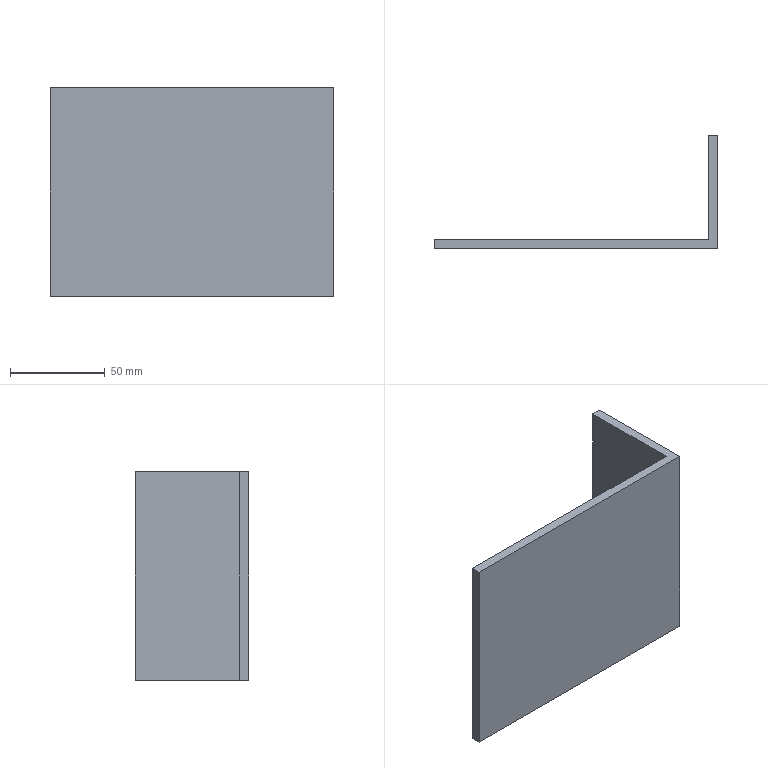Part | SolidWorks | features Extrusion 1 | 1 solid | 8 faces | box 150 x 60 x 110 mm | volume 112750 mm3 | plane 8
STEP:
#1=CARTESIAN_POINT('',(0.,0.,0.));
#2=VERTEX_POINT('',#1);
#3=CARTESIAN_POINT('',(-5.,0.,0.));
#4=VERTEX_POINT('',#3);
#5=CARTESIAN_POINT('',(-5.,0.,0.));
#6=DIRECTION('',(-1.,0.,0.));
#7=VECTOR('',#6,1000.);
#8=LINE('',#5,#7);
#9=EDGE_CURVE('',#2,#4,#8,.T.);
#10=ORIENTED_EDGE('',*,*,#9,.T.);
#11=CARTESIAN_POINT('',(-5.,0.,110.));
#12=VERTEX_POINT('',#11);
#13=CARTESIAN_POINT('',(-5.,0.,110.));
#14=DIRECTION('',(0.,0.,-1.));
#15=VECTOR('',#14,1000.);
#16=LINE('',#13,#15);
#17=EDGE_CURVE('',#12,#4,#16,.T.);
#18=ORIENTED_EDGE('',*,*,#17,.F.);
#19=CARTESIAN_POINT('',(0.,0.,110.));
#20=VERTEX_POINT('',#19);
#21=CARTESIAN_POINT('',(-5.,0.,110.));
#22=DIRECTION('',(-1.,0.,0.));
#23=VECTOR('',#22,1000.);
#24=LINE('',#21,#23);
#25=EDGE_CURVE('',#20,#12,#24,.T.);
#26=ORIENTED_EDGE('',*,*,#25,.F.);
#27=CARTESIAN_POINT('',(0.,0.,110.));
#28=DIRECTION('',(0.,0.,-1.));
#29=VECTOR('',#28,1000.);
#30=LINE('',#27,#29);
#31=EDGE_CURVE('',#20,#2,#30,.T.);
#32=ORIENTED_EDGE('',*,*,#31,.T.);
#33=EDGE_LOOP('',(#10,#18,#26,#32));
#34=FACE_OUTER_BOUND('',#33,.T.);
#35=CARTESIAN_POINT('',(-5.,0.,110.));
#36=DIRECTION('',(0.,-1.,0.));
#37=DIRECTION('',(0.,0.,-1.));
#38=AXIS2_PLACEMENT_3D('',#35,#36,#37);
#39=PLANE('',#38);
#40=ADVANCED_FACE('',(#34),#39,.F.);
#41=CARTESIAN_POINT('',(-5.,-55.,0.));
#42=VERTEX_POINT('',#41);
#43=CARTESIAN_POINT('',(-5.,0.,0.));
#44=DIRECTION('',(0.,-1.,0.));
#45=VECTOR('',#44,1000.);
#46=LINE('',#43,#45);
#47=EDGE_CURVE('',#4,#42,#46,.T.);
#48=ORIENTED_EDGE('',*,*,#47,.T.);
#49=CARTESIAN_POINT('',(-5.,-55.,110.));
#50=VERTEX_POINT('',#49);
#51=CARTESIAN_POINT('',(-5.,-55.,110.));
#52=DIRECTION('',(0.,0.,-1.));
#53=VECTOR('',#52,1000.);
#54=LINE('',#51,#53);
#55=EDGE_CURVE('',#50,#42,#54,.T.);
#56=ORIENTED_EDGE('',*,*,#55,.F.);
#57=CARTESIAN_POINT('',(-5.,0.,110.));
#58=DIRECTION('',(0.,-1.,0.));
#59=VECTOR('',#58,1000.);
#60=LINE('',#57,#59);
#61=EDGE_CURVE('',#12,#50,#60,.T.);
#62=ORIENTED_EDGE('',*,*,#61,.F.);
#63=ORIENTED_EDGE('',*,*,#17,.T.);
#64=EDGE_LOOP('',(#48,#56,#62,#63));
#65=FACE_OUTER_BOUND('',#64,.T.);
#66=CARTESIAN_POINT('',(-5.,0.,110.));
#67=DIRECTION('',(1.,0.,0.));
#68=DIRECTION('',(0.,0.,-1.));
#69=AXIS2_PLACEMENT_3D('',#66,#67,#68);
#70=PLANE('',#69);
#71=ADVANCED_FACE('',(#65),#70,.F.);
#72=CARTESIAN_POINT('',(-150.,-55.,0.));
#73=VERTEX_POINT('',#72);
#74=CARTESIAN_POINT('',(-5.,-55.,0.));
#75=DIRECTION('',(-1.,0.,0.));
#76=VECTOR('',#75,1000.);
#77=LINE('',#74,#76);
#78=EDGE_CURVE('',#42,#73,#77,.T.);
#79=ORIENTED_EDGE('',*,*,#78,.T.);
#80=CARTESIAN_POINT('',(-150.,-55.,110.));
#81=VERTEX_POINT('',#80);
#82=CARTESIAN_POINT('',(-150.,-55.,110.));
#83=DIRECTION('',(0.,0.,-1.));
#84=VECTOR('',#83,1000.);
#85=LINE('',#82,#84);
#86=EDGE_CURVE('',#81,#73,#85,.T.);
#87=ORIENTED_EDGE('',*,*,#86,.F.);
#88=CARTESIAN_POINT('',(-5.,-55.,110.));
#89=DIRECTION('',(-1.,0.,0.));
#90=VECTOR('',#89,1000.);
#91=LINE('',#88,#90);
#92=EDGE_CURVE('',#50,#81,#91,.T.);
#93=ORIENTED_EDGE('',*,*,#92,.F.);
#94=ORIENTED_EDGE('',*,*,#55,.T.);
#95=EDGE_LOOP('',(#79,#87,#93,#94));
#96=FACE_OUTER_BOUND('',#95,.T.);
#97=CARTESIAN_POINT('',(-5.,-55.,110.));
#98=DIRECTION('',(0.,-1.,0.));
#99=DIRECTION('',(0.,0.,-1.));
#100=AXIS2_PLACEMENT_3D('',#97,#98,#99);
#101=PLANE('',#100);
#102=ADVANCED_FACE('',(#96),#101,.F.);
#103=CARTESIAN_POINT('',(-150.,-60.,0.));
#104=VERTEX_POINT('',#103);
#105=CARTESIAN_POINT('',(-150.,-60.,0.));
#106=DIRECTION('',(0.,-1.,0.));
#107=VECTOR('',#106,1000.);
#108=LINE('',#105,#107);
#109=EDGE_CURVE('',#73,#104,#108,.T.);
#110=ORIENTED_EDGE('',*,*,#109,.T.);
#111=CARTESIAN_POINT('',(-150.,-60.,110.));
#112=VERTEX_POINT('',#111);
#113=CARTESIAN_POINT('',(-150.,-60.,110.));
#114=DIRECTION('',(0.,0.,-1.));
#115=VECTOR('',#114,1000.);
#116=LINE('',#113,#115);
#117=EDGE_CURVE('',#112,#104,#116,.T.);
#118=ORIENTED_EDGE('',*,*,#117,.F.);
#119=CARTESIAN_POINT('',(-150.,-60.,110.));
#120=DIRECTION('',(0.,-1.,0.));
#121=VECTOR('',#120,1000.);
#122=LINE('',#119,#121);
#123=EDGE_CURVE('',#81,#112,#122,.T.);
#124=ORIENTED_EDGE('',*,*,#123,.F.);
#125=ORIENTED_EDGE('',*,*,#86,.T.);
#126=EDGE_LOOP('',(#110,#118,#124,#125));
#127=FACE_OUTER_BOUND('',#126,.T.);
#128=CARTESIAN_POINT('',(-150.,-60.,110.));
#129=DIRECTION('',(1.,0.,0.));
#130=DIRECTION('',(0.,0.,-1.));
#131=AXIS2_PLACEMENT_3D('',#128,#129,#130);
#132=PLANE('',#131);
#133=ADVANCED_FACE('',(#127),#132,.F.);
#134=CARTESIAN_POINT('',(0.,-60.,0.));
#135=VERTEX_POINT('',#134);
#136=CARTESIAN_POINT('',(0.,-60.,0.));
#137=DIRECTION('',(1.,0.,0.));
#138=VECTOR('',#137,1000.);
#139=LINE('',#136,#138);
#140=EDGE_CURVE('',#104,#135,#139,.T.);
#141=ORIENTED_EDGE('',*,*,#140,.T.);
#142=CARTESIAN_POINT('',(0.,-60.,110.));
#143=VERTEX_POINT('',#142);
#144=CARTESIAN_POINT('',(0.,-60.,110.));
#145=DIRECTION('',(0.,0.,-1.));
#146=VECTOR('',#145,1000.);
#147=LINE('',#144,#146);
#148=EDGE_CURVE('',#143,#135,#147,.T.);
#149=ORIENTED_EDGE('',*,*,#148,.F.);
#150=CARTESIAN_POINT('',(0.,-60.,110.));
#151=DIRECTION('',(1.,0.,0.));
#152=VECTOR('',#151,1000.);
#153=LINE('',#150,#152);
#154=EDGE_CURVE('',#112,#143,#153,.T.);
#155=ORIENTED_EDGE('',*,*,#154,.F.);
#156=ORIENTED_EDGE('',*,*,#117,.T.);
#157=EDGE_LOOP('',(#141,#149,#155,#156));
#158=FACE_OUTER_BOUND('',#157,.T.);
#159=CARTESIAN_POINT('',(0.,-60.,110.));
#160=DIRECTION('',(0.,1.,0.));
#161=DIRECTION('',(-1.,0.,0.));
#162=AXIS2_PLACEMENT_3D('',#159,#160,#161);
#163=PLANE('',#162);
#164=ADVANCED_FACE('',(#158),#163,.F.);
#165=CARTESIAN_POINT('',(0.,0.,0.));
#166=DIRECTION('',(0.,1.,0.));
#167=VECTOR('',#166,1000.);
#168=LINE('',#165,#167);
#169=EDGE_CURVE('',#135,#2,#168,.T.);
#170=ORIENTED_EDGE('',*,*,#169,.T.);
#171=ORIENTED_EDGE('',*,*,#31,.F.);
#172=CARTESIAN_POINT('',(0.,0.,110.));
#173=DIRECTION('',(0.,1.,0.));
#174=VECTOR('',#173,1000.);
#175=LINE('',#172,#174);
#176=EDGE_CURVE('',#143,#20,#175,.T.);
#177=ORIENTED_EDGE('',*,*,#176,.F.);
#178=ORIENTED_EDGE('',*,*,#148,.T.);
#179=EDGE_LOOP('',(#170,#171,#177,#178));
#180=FACE_OUTER_BOUND('',#179,.T.);
#181=CARTESIAN_POINT('',(0.,0.,110.));
#182=DIRECTION('',(-1.,0.,0.));
#183=DIRECTION('',(0.,-1.,0.));
#184=AXIS2_PLACEMENT_3D('',#181,#182,#183);
#185=PLANE('',#184);
#186=ADVANCED_FACE('',(#180),#185,.F.);
#187=ORIENTED_EDGE('',*,*,#25,.T.);
#188=ORIENTED_EDGE('',*,*,#61,.T.);
#189=ORIENTED_EDGE('',*,*,#92,.T.);
#190=ORIENTED_EDGE('',*,*,#123,.T.);
#191=ORIENTED_EDGE('',*,*,#154,.T.);
#192=ORIENTED_EDGE('',*,*,#176,.T.);
#193=EDGE_LOOP('',(#187,#188,#189,#190,#191,#192));
#194=FACE_OUTER_BOUND('',#193,.T.);
#195=CARTESIAN_POINT('',(0.,0.,110.));
#196=DIRECTION('',(0.,0.,-1.));
#197=DIRECTION('',(-1.,0.,0.));
#198=AXIS2_PLACEMENT_3D('',#195,#196,#197);
#199=PLANE('',#198);
#200=ADVANCED_FACE('',(#194),#199,.F.);
#201=ORIENTED_EDGE('',*,*,#9,.F.);
#202=ORIENTED_EDGE('',*,*,#169,.F.);
#203=ORIENTED_EDGE('',*,*,#140,.F.);
#204=ORIENTED_EDGE('',*,*,#109,.F.);
#205=ORIENTED_EDGE('',*,*,#78,.F.);
#206=ORIENTED_EDGE('',*,*,#47,.F.);
#207=EDGE_LOOP('',(#201,#202,#203,#204,#205,#206));
#208=FACE_OUTER_BOUND('',#207,.T.);
#209=CARTESIAN_POINT('',(0.,0.,0.));
#210=DIRECTION('',(0.,0.,-1.));
#211=DIRECTION('',(-1.,0.,0.));
#212=AXIS2_PLACEMENT_3D('',#209,#210,#211);
#213=PLANE('',#212);
#214=ADVANCED_FACE('',(#208),#213,.T.);
#215=CLOSED_SHELL('',(#40,#71,#102,#133,#164,#186,#200,#214));
#216=MANIFOLD_SOLID_BREP('',#215);
#217=CARTESIAN_POINT('',(0.,0.,0.));
#218=DIRECTION('',(0.,0.,1.));
#219=DIRECTION('',(1.,0.,0.));
#220=AXIS2_PLACEMENT_3D('',#217,#218,#219);
#221=(LENGTH_UNIT()NAMED_UNIT(*)SI_UNIT(.MILLI.,.METRE.));
#222=UNCERTAINTY_MEASURE_WITH_UNIT(LENGTH_MEASURE(0.00001),#221,'','');
#223=(NAMED_UNIT(*)PLANE_ANGLE_UNIT()SI_UNIT($,.RADIAN.));
#224=(NAMED_UNIT(*)SI_UNIT($,.STERADIAN.)SOLID_ANGLE_UNIT());
#225=(GEOMETRIC_REPRESENTATION_CONTEXT(3)GLOBAL_UNCERTAINTY_ASSIGNED_CONTEXT((#222))GLOBAL_UNIT_ASSIGNED_CONTEXT((#221,#223,#224))REPRESENTATION_CONTEXT('',''));
#226=ADVANCED_BREP_SHAPE_REPRESENTATION('',(#216,#220),#225);